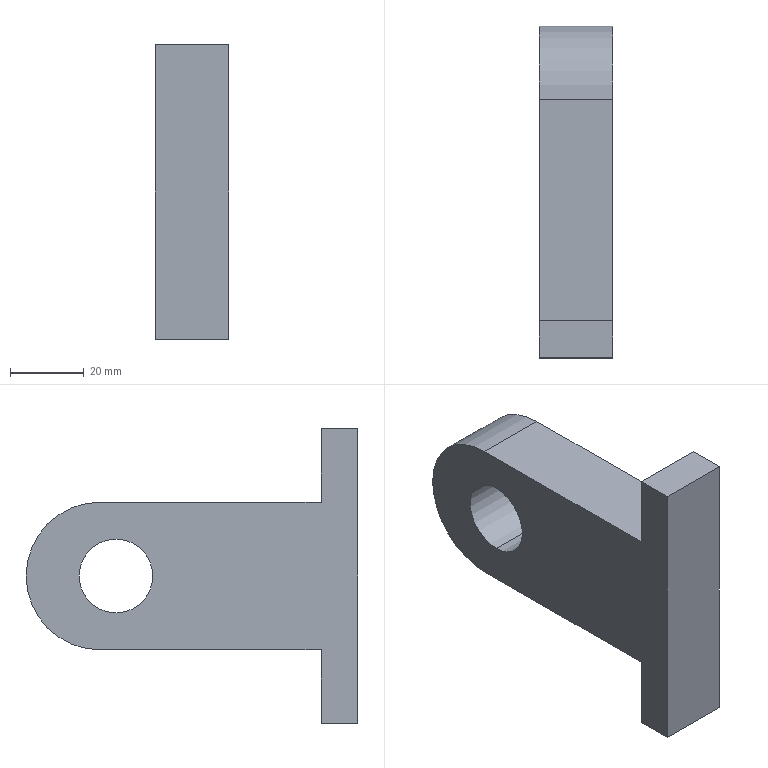Part | SolidWorks | features BaseBody 1 | 1 solid | 13 faces | box 20 x 90 x 80 mm | volume 70283 mm3 | plane 9 | cylinder 4 | commonest cylinder face diameters 20 x2 40 x2
STEP:
#1=CARTESIAN_POINT('',(193.218,72.768,10.));
#2=VERTEX_POINT('',#1);
#3=CARTESIAN_POINT('',(193.218,72.768,-10.));
#4=VERTEX_POINT('',#3);
#5=CARTESIAN_POINT('',(193.218,72.768,0.));
#6=DIRECTION('',(1.,0.,0.));
#7=DIRECTION('',(0.,0.,-1.));
#8=AXIS2_PLACEMENT_3D('',#5,#6,#7);
#9=CIRCLE('',#8,10.);
#10=EDGE_CURVE('',#2,#4,#9,.T.);
#11=ORIENTED_EDGE('',*,*,#10,.F.);
#12=CARTESIAN_POINT('',(213.218,72.768,10.));
#13=VERTEX_POINT('',#12);
#14=CARTESIAN_POINT('',(83.218,72.768,10.));
#15=DIRECTION('',(1.,0.,0.));
#16=VECTOR('',#15,1000.);
#17=LINE('',#14,#16);
#18=EDGE_CURVE('',#2,#13,#17,.T.);
#19=ORIENTED_EDGE('',*,*,#18,.T.);
#20=CARTESIAN_POINT('',(213.218,72.768,-10.));
#21=VERTEX_POINT('',#20);
#22=CARTESIAN_POINT('',(213.218,72.768,0.));
#23=DIRECTION('',(-1.,0.,0.));
#24=DIRECTION('',(0.,0.,1.));
#25=AXIS2_PLACEMENT_3D('',#22,#23,#24);
#26=CIRCLE('',#25,10.);
#27=EDGE_CURVE('',#21,#13,#26,.T.);
#28=ORIENTED_EDGE('',*,*,#27,.F.);
#29=CARTESIAN_POINT('',(83.218,72.768,-10.));
#30=DIRECTION('',(1.,0.,0.));
#31=VECTOR('',#30,1000.);
#32=LINE('',#29,#31);
#33=EDGE_CURVE('',#4,#21,#32,.T.);
#34=ORIENTED_EDGE('',*,*,#33,.F.);
#35=EDGE_LOOP('',(#11,#19,#28,#34));
#36=FACE_OUTER_BOUND('',#35,.T.);
#37=CARTESIAN_POINT('',(83.218,72.768,0.));
#38=DIRECTION('',(1.,0.,0.));
#39=DIRECTION('',(0.,0.,-1.));
#40=AXIS2_PLACEMENT_3D('',#37,#38,#39);
#41=CYLINDRICAL_SURFACE('',#40,10.);
#42=ADVANCED_FACE('',(#36),#41,.F.);
#43=CARTESIAN_POINT('',(193.218,17.138,20.));
#44=VERTEX_POINT('',#43);
#45=CARTESIAN_POINT('',(213.218,17.138,20.));
#46=VERTEX_POINT('',#45);
#47=CARTESIAN_POINT('',(193.218,17.138,20.));
#48=DIRECTION('',(1.,0.,0.));
#49=VECTOR('',#48,1000.);
#50=LINE('',#47,#49);
#51=EDGE_CURVE('',#44,#46,#50,.T.);
#52=ORIENTED_EDGE('',*,*,#51,.F.);
#53=CARTESIAN_POINT('',(193.218,17.138,40.));
#54=VERTEX_POINT('',#53);
#55=CARTESIAN_POINT('',(193.218,17.138,-40.));
#56=DIRECTION('',(0.,0.,1.));
#57=VECTOR('',#56,1000.);
#58=LINE('',#55,#57);
#59=EDGE_CURVE('',#44,#54,#58,.T.);
#60=ORIENTED_EDGE('',*,*,#59,.T.);
#61=CARTESIAN_POINT('',(213.218,17.138,40.));
#62=VERTEX_POINT('',#61);
#63=CARTESIAN_POINT('',(193.218,17.138,40.));
#64=DIRECTION('',(1.,0.,0.));
#65=VECTOR('',#64,1000.);
#66=LINE('',#63,#65);
#67=EDGE_CURVE('',#54,#62,#66,.T.);
#68=ORIENTED_EDGE('',*,*,#67,.T.);
#69=CARTESIAN_POINT('',(213.218,17.138,-40.));
#70=DIRECTION('',(0.,0.,-1.));
#71=VECTOR('',#70,1000.);
#72=LINE('',#69,#71);
#73=EDGE_CURVE('',#62,#46,#72,.T.);
#74=ORIENTED_EDGE('',*,*,#73,.T.);
#75=EDGE_LOOP('',(#52,#60,#68,#74));
#76=FACE_OUTER_BOUND('',#75,.T.);
#77=CARTESIAN_POINT('',(-546.782,17.138,0.));
#78=DIRECTION('',(0.,1.,0.));
#79=DIRECTION('',(0.,0.,1.));
#80=AXIS2_PLACEMENT_3D('',#77,#78,#79);
#81=PLANE('',#80);
#82=ADVANCED_FACE('',(#76),#81,.T.);
#83=CARTESIAN_POINT('',(213.218,77.138,20.));
#84=VERTEX_POINT('',#83);
#85=CARTESIAN_POINT('',(213.218,97.138,20.));
#86=DIRECTION('',(0.,-1.,0.));
#87=VECTOR('',#86,1000.);
#88=LINE('',#85,#87);
#89=EDGE_CURVE('',#84,#46,#88,.T.);
#90=ORIENTED_EDGE('',*,*,#89,.F.);
#91=CARTESIAN_POINT('',(193.218,77.138,20.));
#92=VERTEX_POINT('',#91);
#93=CARTESIAN_POINT('',(193.218,77.138,20.));
#94=DIRECTION('',(-1.,0.,0.));
#95=VECTOR('',#94,1000.);
#96=LINE('',#93,#95);
#97=EDGE_CURVE('',#84,#92,#96,.T.);
#98=ORIENTED_EDGE('',*,*,#97,.T.);
#99=CARTESIAN_POINT('',(193.218,97.138,20.));
#100=DIRECTION('',(0.,-1.,0.));
#101=VECTOR('',#100,1000.);
#102=LINE('',#99,#101);
#103=EDGE_CURVE('',#92,#44,#102,.T.);
#104=ORIENTED_EDGE('',*,*,#103,.T.);
#105=ORIENTED_EDGE('',*,*,#51,.T.);
#106=EDGE_LOOP('',(#90,#98,#104,#105));
#107=FACE_OUTER_BOUND('',#106,.T.);
#108=CARTESIAN_POINT('',(193.218,97.138,20.));
#109=DIRECTION('',(0.,0.,-1.));
#110=DIRECTION('',(-1.,0.,0.));
#111=AXIS2_PLACEMENT_3D('',#108,#109,#110);
#112=PLANE('',#111);
#113=ADVANCED_FACE('',(#107),#112,.F.);
#114=ORIENTED_EDGE('',*,*,#97,.F.);
#115=CARTESIAN_POINT('',(213.218,97.138,0.));
#116=VERTEX_POINT('',#115);
#117=CARTESIAN_POINT('',(213.218,77.138,0.));
#118=DIRECTION('',(1.,0.,0.));
#119=DIRECTION('',(0.,0.,1.));
#120=AXIS2_PLACEMENT_3D('',#117,#118,#119);
#121=CIRCLE('',#120,20.);
#122=EDGE_CURVE('',#116,#84,#121,.T.);
#123=ORIENTED_EDGE('',*,*,#122,.F.);
#124=CARTESIAN_POINT('',(193.218,97.138,0.));
#125=VERTEX_POINT('',#124);
#126=CARTESIAN_POINT('',(213.218,97.138,0.));
#127=DIRECTION('',(1.,0.,0.));
#128=VECTOR('',#127,1000.);
#129=LINE('',#126,#128);
#130=EDGE_CURVE('',#125,#116,#129,.T.);
#131=ORIENTED_EDGE('',*,*,#130,.F.);
#132=CARTESIAN_POINT('',(193.218,77.138,0.));
#133=DIRECTION('',(-1.,0.,0.));
#134=DIRECTION('',(0.,0.,-1.));
#135=AXIS2_PLACEMENT_3D('',#132,#133,#134);
#136=CIRCLE('',#135,20.);
#137=EDGE_CURVE('',#92,#125,#136,.T.);
#138=ORIENTED_EDGE('',*,*,#137,.F.);
#139=EDGE_LOOP('',(#114,#123,#131,#138));
#140=FACE_OUTER_BOUND('',#139,.T.);
#141=CARTESIAN_POINT('',(-546.782,77.138,0.));
#142=DIRECTION('',(-1.,0.,0.));
#143=DIRECTION('',(0.,0.,1.));
#144=AXIS2_PLACEMENT_3D('',#141,#142,#143);
#145=CYLINDRICAL_SURFACE('',#144,20.);
#146=ADVANCED_FACE('',(#140),#145,.T.);
#147=CARTESIAN_POINT('',(213.218,77.138,-20.));
#148=VERTEX_POINT('',#147);
#149=CARTESIAN_POINT('',(213.218,77.138,0.));
#150=DIRECTION('',(1.,0.,0.));
#151=DIRECTION('',(0.,0.,1.));
#152=AXIS2_PLACEMENT_3D('',#149,#150,#151);
#153=CIRCLE('',#152,20.);
#154=EDGE_CURVE('',#148,#116,#153,.T.);
#155=ORIENTED_EDGE('',*,*,#154,.F.);
#156=CARTESIAN_POINT('',(193.218,77.138,-20.));
#157=VERTEX_POINT('',#156);
#158=CARTESIAN_POINT('',(213.218,77.138,-20.));
#159=DIRECTION('',(1.,0.,0.));
#160=VECTOR('',#159,1000.);
#161=LINE('',#158,#160);
#162=EDGE_CURVE('',#157,#148,#161,.T.);
#163=ORIENTED_EDGE('',*,*,#162,.F.);
#164=CARTESIAN_POINT('',(193.218,77.138,0.));
#165=DIRECTION('',(-1.,0.,0.));
#166=DIRECTION('',(0.,0.,-1.));
#167=AXIS2_PLACEMENT_3D('',#164,#165,#166);
#168=CIRCLE('',#167,20.);
#169=EDGE_CURVE('',#125,#157,#168,.T.);
#170=ORIENTED_EDGE('',*,*,#169,.F.);
#171=ORIENTED_EDGE('',*,*,#130,.T.);
#172=EDGE_LOOP('',(#155,#163,#170,#171));
#173=FACE_OUTER_BOUND('',#172,.T.);
#174=CARTESIAN_POINT('',(-546.782,77.138,0.));
#175=DIRECTION('',(1.,0.,0.));
#176=DIRECTION('',(0.,0.,-1.));
#177=AXIS2_PLACEMENT_3D('',#174,#175,#176);
#178=CYLINDRICAL_SURFACE('',#177,20.);
#179=ADVANCED_FACE('',(#173),#178,.T.);
#180=CARTESIAN_POINT('',(193.218,17.138,-20.));
#181=VERTEX_POINT('',#180);
#182=CARTESIAN_POINT('',(193.218,97.138,-20.));
#183=DIRECTION('',(0.,-1.,0.));
#184=VECTOR('',#183,1000.);
#185=LINE('',#182,#184);
#186=EDGE_CURVE('',#157,#181,#185,.T.);
#187=ORIENTED_EDGE('',*,*,#186,.F.);
#188=ORIENTED_EDGE('',*,*,#162,.T.);
#189=CARTESIAN_POINT('',(213.218,17.138,-20.));
#190=VERTEX_POINT('',#189);
#191=CARTESIAN_POINT('',(213.218,97.138,-20.));
#192=DIRECTION('',(0.,-1.,0.));
#193=VECTOR('',#192,1000.);
#194=LINE('',#191,#193);
#195=EDGE_CURVE('',#148,#190,#194,.T.);
#196=ORIENTED_EDGE('',*,*,#195,.T.);
#197=CARTESIAN_POINT('',(193.218,17.138,-20.));
#198=DIRECTION('',(-1.,0.,0.));
#199=VECTOR('',#198,1000.);
#200=LINE('',#197,#199);
#201=EDGE_CURVE('',#190,#181,#200,.T.);
#202=ORIENTED_EDGE('',*,*,#201,.T.);
#203=EDGE_LOOP('',(#187,#188,#196,#202));
#204=FACE_OUTER_BOUND('',#203,.T.);
#205=CARTESIAN_POINT('',(193.218,97.138,-20.));
#206=DIRECTION('',(0.,0.,1.));
#207=DIRECTION('',(1.,0.,0.));
#208=AXIS2_PLACEMENT_3D('',#205,#206,#207);
#209=PLANE('',#208);
#210=ADVANCED_FACE('',(#204),#209,.F.);
#211=ORIENTED_EDGE('',*,*,#18,.F.);
#212=CARTESIAN_POINT('',(193.218,72.768,0.));
#213=DIRECTION('',(1.,0.,0.));
#214=DIRECTION('',(0.,0.,-1.));
#215=AXIS2_PLACEMENT_3D('',#212,#213,#214);
#216=CIRCLE('',#215,10.);
#217=EDGE_CURVE('',#4,#2,#216,.T.);
#218=ORIENTED_EDGE('',*,*,#217,.F.);
#219=ORIENTED_EDGE('',*,*,#33,.T.);
#220=CARTESIAN_POINT('',(213.218,72.768,0.));
#221=DIRECTION('',(-1.,0.,0.));
#222=DIRECTION('',(0.,0.,1.));
#223=AXIS2_PLACEMENT_3D('',#220,#221,#222);
#224=CIRCLE('',#223,10.);
#225=EDGE_CURVE('',#13,#21,#224,.T.);
#226=ORIENTED_EDGE('',*,*,#225,.F.);
#227=EDGE_LOOP('',(#211,#218,#219,#226));
#228=FACE_OUTER_BOUND('',#227,.T.);
#229=CARTESIAN_POINT('',(83.218,72.768,0.));
#230=DIRECTION('',(1.,0.,0.));
#231=DIRECTION('',(0.,0.,-1.));
#232=AXIS2_PLACEMENT_3D('',#229,#230,#231);
#233=CYLINDRICAL_SURFACE('',#232,10.);
#234=ADVANCED_FACE('',(#228),#233,.F.);
#235=ORIENTED_EDGE('',*,*,#201,.F.);
#236=CARTESIAN_POINT('',(213.218,17.138,-40.));
#237=VERTEX_POINT('',#236);
#238=CARTESIAN_POINT('',(213.218,17.138,-40.));
#239=DIRECTION('',(0.,0.,-1.));
#240=VECTOR('',#239,1000.);
#241=LINE('',#238,#240);
#242=EDGE_CURVE('',#190,#237,#241,.T.);
#243=ORIENTED_EDGE('',*,*,#242,.T.);
#244=CARTESIAN_POINT('',(193.218,17.138,-40.));
#245=VERTEX_POINT('',#244);
#246=CARTESIAN_POINT('',(193.218,17.138,-40.));
#247=DIRECTION('',(-1.,0.,0.));
#248=VECTOR('',#247,1000.);
#249=LINE('',#246,#248);
#250=EDGE_CURVE('',#237,#245,#249,.T.);
#251=ORIENTED_EDGE('',*,*,#250,.T.);
#252=CARTESIAN_POINT('',(193.218,17.138,-40.));
#253=DIRECTION('',(0.,0.,1.));
#254=VECTOR('',#253,1000.);
#255=LINE('',#252,#254);
#256=EDGE_CURVE('',#245,#181,#255,.T.);
#257=ORIENTED_EDGE('',*,*,#256,.T.);
#258=EDGE_LOOP('',(#235,#243,#251,#257));
#259=FACE_OUTER_BOUND('',#258,.T.);
#260=CARTESIAN_POINT('',(-546.782,17.138,0.));
#261=DIRECTION('',(0.,1.,0.));
#262=DIRECTION('',(0.,0.,1.));
#263=AXIS2_PLACEMENT_3D('',#260,#261,#262);
#264=PLANE('',#263);
#265=ADVANCED_FACE('',(#259),#264,.T.);
#266=CARTESIAN_POINT('',(213.218,7.138,-40.));
#267=VERTEX_POINT('',#266);
#268=CARTESIAN_POINT('',(193.218,7.138,-40.));
#269=VERTEX_POINT('',#268);
#270=CARTESIAN_POINT('',(193.218,7.138,-40.));
#271=DIRECTION('',(-1.,0.,0.));
#272=VECTOR('',#271,1000.);
#273=LINE('',#270,#272);
#274=EDGE_CURVE('',#267,#269,#273,.T.);
#275=ORIENTED_EDGE('',*,*,#274,.T.);
#276=CARTESIAN_POINT('',(193.218,17.138,-40.));
#277=DIRECTION('',(0.,-1.,0.));
#278=VECTOR('',#277,1000.);
#279=LINE('',#276,#278);
#280=EDGE_CURVE('',#245,#269,#279,.T.);
#281=ORIENTED_EDGE('',*,*,#280,.F.);
#282=ORIENTED_EDGE('',*,*,#250,.F.);
#283=CARTESIAN_POINT('',(213.218,17.138,-40.));
#284=DIRECTION('',(0.,-1.,0.));
#285=VECTOR('',#284,1000.);
#286=LINE('',#283,#285);
#287=EDGE_CURVE('',#237,#267,#286,.T.);
#288=ORIENTED_EDGE('',*,*,#287,.T.);
#289=EDGE_LOOP('',(#275,#281,#282,#288));
#290=FACE_OUTER_BOUND('',#289,.T.);
#291=CARTESIAN_POINT('',(193.218,17.138,-40.));
#292=DIRECTION('',(0.,0.,1.));
#293=DIRECTION('',(1.,0.,0.));
#294=AXIS2_PLACEMENT_3D('',#291,#292,#293);
#295=PLANE('',#294);
#296=ADVANCED_FACE('',(#290),#295,.F.);
#297=ORIENTED_EDGE('',*,*,#27,.T.);
#298=ORIENTED_EDGE('',*,*,#225,.T.);
#299=EDGE_LOOP('',(#297,#298));
#300=FACE_BOUND('',#299,.T.);
#301=ORIENTED_EDGE('',*,*,#195,.F.);
#302=ORIENTED_EDGE('',*,*,#154,.T.);
#303=ORIENTED_EDGE('',*,*,#122,.T.);
#304=ORIENTED_EDGE('',*,*,#89,.T.);
#305=ORIENTED_EDGE('',*,*,#73,.F.);
#306=CARTESIAN_POINT('',(213.218,7.138,40.));
#307=VERTEX_POINT('',#306);
#308=CARTESIAN_POINT('',(213.218,17.138,40.));
#309=DIRECTION('',(0.,-1.,0.));
#310=VECTOR('',#309,1000.);
#311=LINE('',#308,#310);
#312=EDGE_CURVE('',#62,#307,#311,.T.);
#313=ORIENTED_EDGE('',*,*,#312,.T.);
#314=CARTESIAN_POINT('',(213.218,7.138,-40.));
#315=DIRECTION('',(0.,0.,-1.));
#316=VECTOR('',#315,1000.);
#317=LINE('',#314,#316);
#318=EDGE_CURVE('',#307,#267,#317,.T.);
#319=ORIENTED_EDGE('',*,*,#318,.T.);
#320=ORIENTED_EDGE('',*,*,#287,.F.);
#321=ORIENTED_EDGE('',*,*,#242,.F.);
#322=EDGE_LOOP('',(#301,#302,#303,#304,#305,#313,#319,#320,#321));
#323=FACE_OUTER_BOUND('',#322,.T.);
#324=CARTESIAN_POINT('',(213.218,17.138,-40.));
#325=DIRECTION('',(-1.,0.,0.));
#326=DIRECTION('',(0.,0.,1.));
#327=AXIS2_PLACEMENT_3D('',#324,#325,#326);
#328=PLANE('',#327);
#329=ADVANCED_FACE('',(#300,#323),#328,.F.);
#330=CARTESIAN_POINT('',(193.218,7.138,40.));
#331=VERTEX_POINT('',#330);
#332=CARTESIAN_POINT('',(193.218,7.138,40.));
#333=DIRECTION('',(1.,0.,0.));
#334=VECTOR('',#333,1000.);
#335=LINE('',#332,#334);
#336=EDGE_CURVE('',#331,#307,#335,.T.);
#337=ORIENTED_EDGE('',*,*,#336,.T.);
#338=ORIENTED_EDGE('',*,*,#312,.F.);
#339=ORIENTED_EDGE('',*,*,#67,.F.);
#340=CARTESIAN_POINT('',(193.218,17.138,40.));
#341=DIRECTION('',(0.,-1.,0.));
#342=VECTOR('',#341,1000.);
#343=LINE('',#340,#342);
#344=EDGE_CURVE('',#54,#331,#343,.T.);
#345=ORIENTED_EDGE('',*,*,#344,.T.);
#346=EDGE_LOOP('',(#337,#338,#339,#345));
#347=FACE_OUTER_BOUND('',#346,.T.);
#348=CARTESIAN_POINT('',(193.218,17.138,40.));
#349=DIRECTION('',(0.,0.,-1.));
#350=DIRECTION('',(-1.,0.,0.));
#351=AXIS2_PLACEMENT_3D('',#348,#349,#350);
#352=PLANE('',#351);
#353=ADVANCED_FACE('',(#347),#352,.F.);
#354=ORIENTED_EDGE('',*,*,#217,.T.);
#355=ORIENTED_EDGE('',*,*,#10,.T.);
#356=EDGE_LOOP('',(#354,#355));
#357=FACE_BOUND('',#356,.T.);
#358=ORIENTED_EDGE('',*,*,#137,.T.);
#359=ORIENTED_EDGE('',*,*,#169,.T.);
#360=ORIENTED_EDGE('',*,*,#186,.T.);
#361=ORIENTED_EDGE('',*,*,#256,.F.);
#362=ORIENTED_EDGE('',*,*,#280,.T.);
#363=CARTESIAN_POINT('',(193.218,7.138,-40.));
#364=DIRECTION('',(0.,0.,1.));
#365=VECTOR('',#364,1000.);
#366=LINE('',#363,#365);
#367=EDGE_CURVE('',#269,#331,#366,.T.);
#368=ORIENTED_EDGE('',*,*,#367,.T.);
#369=ORIENTED_EDGE('',*,*,#344,.F.);
#370=ORIENTED_EDGE('',*,*,#59,.F.);
#371=ORIENTED_EDGE('',*,*,#103,.F.);
#372=EDGE_LOOP('',(#358,#359,#360,#361,#362,#368,#369,#370,#371));
#373=FACE_OUTER_BOUND('',#372,.T.);
#374=CARTESIAN_POINT('',(193.218,17.138,-40.));
#375=DIRECTION('',(1.,0.,0.));
#376=DIRECTION('',(0.,0.,-1.));
#377=AXIS2_PLACEMENT_3D('',#374,#375,#376);
#378=PLANE('',#377);
#379=ADVANCED_FACE('',(#357,#373),#378,.F.);
#380=ORIENTED_EDGE('',*,*,#274,.F.);
#381=ORIENTED_EDGE('',*,*,#318,.F.);
#382=ORIENTED_EDGE('',*,*,#336,.F.);
#383=ORIENTED_EDGE('',*,*,#367,.F.);
#384=EDGE_LOOP('',(#380,#381,#382,#383));
#385=FACE_OUTER_BOUND('',#384,.T.);
#386=CARTESIAN_POINT('',(28.218,7.138,0.));
#387=DIRECTION('',(0.,1.,0.));
#388=DIRECTION('',(0.,0.,1.));
#389=AXIS2_PLACEMENT_3D('',#386,#387,#388);
#390=PLANE('',#389);
#391=ADVANCED_FACE('',(#385),#390,.F.);
#392=CLOSED_SHELL('',(#42,#82,#113,#146,#179,#210,#234,#265,#296,#329,#353,#379,#391));
#393=MANIFOLD_SOLID_BREP('',#392);
#394=CARTESIAN_POINT('',(0.,0.,0.));
#395=DIRECTION('',(0.,0.,1.));
#396=DIRECTION('',(1.,0.,0.));
#397=AXIS2_PLACEMENT_3D('',#394,#395,#396);
#398=(LENGTH_UNIT()NAMED_UNIT(*)SI_UNIT(.MILLI.,.METRE.));
#399=UNCERTAINTY_MEASURE_WITH_UNIT(LENGTH_MEASURE(0.00001),#398,'','');
#400=(NAMED_UNIT(*)PLANE_ANGLE_UNIT()SI_UNIT($,.RADIAN.));
#401=(NAMED_UNIT(*)SI_UNIT($,.STERADIAN.)SOLID_ANGLE_UNIT());
#402=(GEOMETRIC_REPRESENTATION_CONTEXT(3)GLOBAL_UNCERTAINTY_ASSIGNED_CONTEXT((#399))GLOBAL_UNIT_ASSIGNED_CONTEXT((#398,#400,#401))REPRESENTATION_CONTEXT('',''));
#403=ADVANCED_BREP_SHAPE_REPRESENTATION('',(#393,#397),#402);